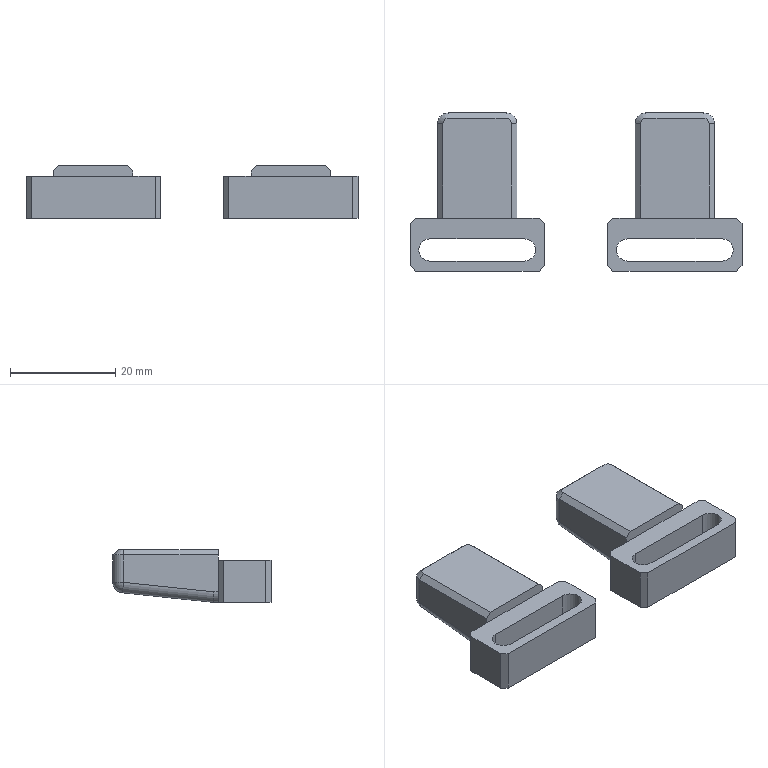NC program | NX | posted with a generic post | part box 63 x 30 x 10 mm
Lines 137 to 1195 of 24780:
(FIXED_CONTOUR , TOOL : D4R0.5)
N260 T16 M6
N262 G54
N264 G17 G0 G90 X-28.436 Y-13.585 B0. C0. S9500 M3
N266 G43 Z30. H16
N268 Z1.2
N270 G94 G1 Z-4.301 F1000.
N272 G3 X-28.236 Y-13.239 R0.4
N274 G1 Y-13.205 Z-4.212 F2500.
N276 X-28.242 Y-13.128 Z-4.201
N278 X-28.244 Y-12.729 Z-4.164
N280 X-28.245 Y1.946 Z-2.62
N282 X-28.246 Y2.589 Z-2.552
N284 X-28.245 Y2.666 Z-2.533
N286 X-28.243 Y2.712 Z-2.504
N288 X-28.238 Y2.806 Z-2.428
N290 X-28.236 Y2.911 Z-2.402
N292 Y2.92 Z-2.427
N294 Y2.921 Z-2.368
N296 Z-2.37
N298 Y2.939 Z-2.373
N300 Y2.944 Z-2.365
N302 Y2.961 Z-2.371
N304 Y2.981 Z-2.369
N306 Y2.999 Z-2.393
N308 Z-2.388
N310 Z-2.393
N312 Y2.981 Z-2.369
N314 Y2.961 Z-2.371
N316 Y2.944 Z-2.365
N318 Y2.939 Z-2.373
N320 Y2.921 Z-2.37
N322 Z-2.368
N324 Y2.92 Z-2.427
N326 Y2.911 Z-2.402
N328 X-28.238 Y2.806 Z-2.428
N330 Y0.416 Z-2.693
N332 Y-0.584 Z-2.805
N334 Y-3.37 Z-3.107
N336 Y-12.729 Z-4.086
N338 Y-12.885 Z-4.117
N340 Y-13.128 Z-4.155
N342 Y-13.177 Z-4.208
N344 X-28.236 Y-13.205 Z-4.212
N346 Y-13.239 Z-4.301
N348 X-28.231 Y-13.303
N350 Y-13.271 Z-4.215
N352 Y-13.128 Z-4.06
N354 Y-13.016 Z-4.042
N356 Y-12.729 Z-3.986
N358 X-28.23 Y-3.169 Z-2.996
N360 Y0.846 Z-2.545
N362 Y2.806 Z-2.334
N364 Y2.959
N366 Y2.963 Z-2.345
N368 Y2.964 Z-2.312
N370 Y2.982 Z-2.32
N372 Y2.991 Z-2.319
N374 Y2.999 Z-2.329
N376 X-28.226 Z-2.279
N378 X-28.221 Z-2.254
N380 Y2.94 Z-2.257
N382 Y0.251 Z-2.543
N384 Y-3.331 Z-2.934
N386 X-28.222 Y-11.136 Z-3.744
N388 Y-12.729 Z-3.91
N390 Y-13.128 Z-3.96
N392 Y-13.163 Z-3.981
N394 Y-13.383 Z-4.219
N396 Y-13.412 Z-4.301
N398 X-28.212 Y-13.528
N400 Y-13.526 Z-4.287
N402 Y-13.505 Z-4.224
N404 Y-13.293 Z-3.99
N406 Y-13.128 Z-3.89
N408 Y-12.729 Z-3.842
N410 X-28.211 Y-11.506 Z-3.713
N412 Y-8.746 Z-3.421
N414 Y2.815 Z-2.214
N416 Y2.999 Z-2.203
N418 X-28.2 Z-2.139
N420 Z-2.147
N422 Y2.806 Z-2.158
N424 Y-10.443 Z-3.545
N426 X-28.201 Y-12.434 Z-3.757
N428 Y-12.823 Z-3.798
N430 Y-13.128 Z-3.827
N432 Y-13.204 Z-3.859
N434 Y-13.436 Z-4.
N436 Y-13.526 Z-4.1
N438 Y-13.564 Z-4.2
N440 Y-13.576 Z-4.224
N442 Y-13.588 Z-4.301
N444 X-28.186 Y-13.667
N446 Y-13.655 Z-4.223
N448 Y-13.624 Z-4.16
N450 Y-13.563 Z-4.001
N452 Y-13.526 Z-3.952
N454 Y-13.405 Z-3.878
N456 Y-13.128 Z-3.761
N458 Y-12.965 Z-3.745
N460 Y-12.59 Z-3.705
N462 Y-5.957 Z-3.004
N464 X-28.185 Y2.806 Z-2.083
N466 Y2.999 Z-2.074
N468 Z-2.068
N470 X-28.167 Y2.998 Z-1.981
N472 Y2.806 Z-2.
N474 X-28.168 Y-12.729 Z-3.641
N476 Y-13.128 Z-3.68
N478 Y-13.155 Z-3.689
N480 Y-13.526 Z-3.844
N482 Y-13.555 Z-3.871
N484 Y-13.57 Z-3.882
N486 Y-13.654 Z-3.991
N488 Y-13.699 Z-4.11
N490 Y-13.754 Z-4.222
N492 Y-13.766 Z-4.301
N494 X-28.15 Y-13.865
N496 Y-13.853 Z-4.22
N498 Y-13.775 Z-4.06
N500 Y-13.744 Z-3.981
N502 Y-13.699 Z-3.92
N504 Y-13.653 Z-3.866
N506 Y-13.609 Z-3.835
N508 X-28.149 Y-13.526 Z-3.756
N510 Y-13.451 Z-3.724
N512 Y-13.128 Z-3.622
N514 Y-11.534 Z-3.456
N516 Y-3.368 Z-2.594
N518 Y2.998 Z-1.921
N520 X-28.129 Z-1.856
N522 Y-9.543 Z-3.183
N524 Y-13.128 Z-3.558
N526 Y-13.401 Z-3.645
N528 X-28.13 Y-13.526 Z-3.68
N530 Y-13.586 Z-3.717
N532 Y-13.668 Z-3.795
N534 Y-13.744 Z-3.849
N536 Y-13.823 Z-3.942
N538 Y-13.843 Z-3.97
N540 Y-13.857 Z-4.005
N542 Y-13.925 Z-4.143
N544 Y-13.948 Z-4.22
N546 Y-13.955 Z-4.3
N548 X-28.107 Y-14.03 Z-4.301
N550 Y-14.023 Z-4.222
N552 Y-14.01 Z-4.173
N554 Y-13.942 Z-3.957
N556 Y-13.925 Z-3.925
N558 Y-13.844 Z-3.831
N560 Y-13.734 Z-3.751
N562 Y-13.673 Z-3.693
N564 Y-13.526 Z-3.602
N566 Y-13.219 Z-3.517
N568 Y-13.128 Z-3.488
N570 Y-7.7 Z-2.92
N572 Y2.998 Z-1.785
N574 X-28.087 Y2.999 Z-1.74
N576 X-28.079 Z-1.717
N578 Z-1.722
N580 Y2.935 Z-1.723
N582 Y2.806 Z-1.732
N584 X-28.08 Y-9.144 Z-2.996
N586 Y-13.128 Z-3.412
N588 Y-13.526 Z-3.507
N590 Y-13.779 Z-3.664
N592 Y-13.814 Z-3.697
N594 Y-13.925 Z-3.776
N596 Y-13.961 Z-3.822
N598 Y-14.042 Z-3.973
N600 Y-14.091 Z-4.129
N602 Y-14.116 Z-4.224
N604 Y-14.123 Z-4.301
N606 X-28.052 Y-14.219
N608 Y-14.211 Z-4.226
N610 Y-14.174 Z-4.084
N612 Y-14.143 Z-3.984
N614 Y-14.114 Z-3.925
N616 Y-14.067 Z-3.841
N618 Y-14.032 Z-3.792
N620 Y-13.925 Z-3.66
N622 Y-13.89 Z-3.633
N624 Y-13.828 Z-3.595
N626 Y-13.569 Z-3.453
N628 Y-13.526 Z-3.432
N630 Y-13.331 Z-3.389
N632 Y-13.128 Z-3.34
N634 Y-6.5 Z-2.644
N636 X-28.051 Y2.806 Z-1.663
N638 Y2.87 Z-1.658
N640 Y2.999 Z-1.656
N642 Z-1.634
N644 X-28.023 Z-1.581
N646 Z-1.591
N648 Y2.809 Z-1.593
N650 X-28.024 Y-13.128 Z-3.269
N652 Y-13.526 Z-3.358
N654 Y-13.612 Z-3.399
N656 Y-13.698 Z-3.444
N658 Y-13.945 Z-3.581
N660 Y-13.986 Z-3.618
N662 Y-14.112 Z-3.775
N664 Y-14.174 Z-3.86
N666 Y-14.201 Z-3.909
N668 Y-14.244 Z-3.995
N670 Y-14.258 Z-4.039
N672 Y-14.307 Z-4.229
N674 Y-14.314 Z-4.3
N676 X-27.993 Y-14.399 Z-4.301
N678 Y-14.395 Z-4.24
N680 Y-14.386 Z-4.17
N682 Y-14.35 Z-4.015
N684 Y-14.323 Z-3.947
N686 Y-14.289 Z-3.88
N688 Y-14.199 Z-3.756
N690 Y-14.136 Z-3.679
N692 Y-14.083 Z-3.61
N694 Y-14.03 Z-3.559
N696 Y-13.977 Z-3.515
N698 Y-13.791 Z-3.41
N700 Y-13.658 Z-3.342
N702 Y-13.592 Z-3.309
N704 Y-13.526 Z-3.286
N706 Y-13.208 Z-3.217
N708 Y2.888 Z-1.522
N710 Y2.999 Z-1.521
N712 X-27.96 Z-1.445
N714 Y2.973
N716 X-27.961 Y-13.128 Z-3.142
N718 Y-13.297 Z-3.161
N720 Y-13.526 Z-3.213
N722 Y-13.692 Z-3.271
N724 Y-13.925 Z-3.392
N726 Y-14.012 Z-3.444
N728 Y-14.1 Z-3.516
N730 Y-14.188 Z-3.6
N732 Y-14.323 Z-3.778
N734 Y-14.389 Z-3.883
N736 Y-14.438 Z-4.003
N738 Y-14.457 Z-4.057
N740 Y-14.466 Z-4.096
N742 Y-14.487 Z-4.264
N744 Y-14.489 Z-4.301
N746 X-27.95 Y-14.519
N748 X-27.921 Y-14.581
N750 Y-14.578 Z-4.247
N752 Y-14.561 Z-4.117
N754 Y-14.549 Z-4.053
N756 Y-14.522 Z-3.976
N758 Y-14.484 Z-3.88
N760 Y-14.47 Z-3.853
N762 Y-14.389 Z-3.726
N764 Y-14.323 Z-3.63
N766 Y-14.28 Z-3.573
N768 Y-14.18 Z-3.477
N770 Y-14.109 Z-3.418
N772 Y-14.066 Z-3.389
N774 Y-13.996 Z-3.344
N776 Y-13.925 Z-3.302
N778 Y-13.782 Z-3.228
N780 Y-13.526 Z-3.138
N782 Y-13.383 Z-3.105
N784 Y-13.271 Z-3.088
N786 Y2.944 Z-1.378
N788 Y2.999 Z-1.376
N790 X-27.894 Z-1.333
N792 X-27.879 Z-1.306
N794 Z-1.311
N796 Y2.863 Z-1.316
N798 X-27.88 Y-13.188 Z-3.006
N800 Y-13.466 Z-3.05
N802 Y-13.526 Z-3.064
N804 Y-13.864 Z-3.183
N806 Y-13.925 Z-3.214
N808 Y-14.128 Z-3.342
N810 Y-14.233 Z-3.415
N812 Y-14.263 Z-3.44
N814 Y-14.323 Z-3.498
N816 Y-14.363 Z-3.547
N818 Y-14.388 Z-3.58
N820 Y-14.486 Z-3.722
N822 Y-14.543 Z-3.813
N824 Y-14.578 Z-3.877
N826 Y-14.601 Z-3.935
N828 Y-14.633 Z-4.026
N830 Y-14.661 Z-4.184
N832 Y-14.668 Z-4.233
N834 Y-14.671 Z-4.301
N836 X-27.857 Y-14.721
N838 X-27.837 Y-14.757
N840 Y-14.753 Z-4.223
N842 Y-14.718 Z-3.999
N844 Y-14.675 Z-3.875
N846 Y-14.618 Z-3.771
N848 Y-14.585 Z-3.719
N850 Y-14.528 Z-3.636
N852 Y-14.449 Z-3.53
N854 Y-14.356 Z-3.419
N856 Y-14.323 Z-3.386
N858 Y-14.192 Z-3.294
N860 Y-13.974 Z-3.156
N862 Y-13.925 Z-3.129
N864 Y-13.575 Z-3.006
N866 Y-13.526 Z-2.991
N868 Y-13.128 Z-2.929
N870 Y2.832 Z-1.251
N872 Y2.999 Z-1.244
N874 Z-1.238
N876 X-27.792 Z-1.175
N878 Y2.918 Z-1.178
N880 X-27.793 Y-13.128 Z-2.864
N882 Y-13.241 Z-2.885
N884 Y-13.354 Z-2.898
N886 Y-13.526 Z-2.925
N888 Y-13.752 Z-2.991
N890 Y-13.925 Z-3.053
N892 Y-14.15 Z-3.176
N894 Y-14.258 Z-3.244
N896 Y-14.323 Z-3.29
N898 Y-14.424 Z-3.385
N900 Y-14.476 Z-3.438
N902 Y-14.538 Z-3.513
N904 Y-14.688 Z-3.715
N906 Y-14.721 Z-3.773
N908 Y-14.764 Z-3.871
N910 Y-14.799 Z-3.995
N912 Y-14.834 Z-4.221
N914 Y-14.838 Z-4.301
N916 X-27.746 Y-14.925
N918 Y-14.921 Z-4.219
N920 Y-14.884 Z-3.992
N922 Y-14.848 Z-3.866
N924 Y-14.828 Z-3.824
N926 Y-14.779 Z-3.71
N928 Y-14.721 Z-3.611
N930 Y-14.634 Z-3.494
N932 Y-14.605 Z-3.459
N934 X-27.745 Y-14.509 Z-3.362
N936 Y-14.331 Z-3.195
N938 Y-14.323 Z-3.188
N940 Y-13.925 Z-2.972
N942 Y-13.526 Z-2.854
N944 Y-13.336 Z-2.833
N946 Y-13.128 Z-2.795
N948 Y2.998 Z-1.102
N950 X-27.697 Y2.999 Z-1.044
N952 Y-13.128 Z-2.738
N954 Y-13.337 Z-2.763
N956 Y-13.431 Z-2.78
N958 Y-13.526 Z-2.791
N960 Y-13.735 Z-2.847
N962 Y-13.925 Z-2.903
N964 Y-14.133 Z-3.002
N966 Y-14.323 Z-3.106
N968 Y-14.427 Z-3.185
N970 Y-14.492 Z-3.241
N972 Y-14.594 Z-3.338
N974 Y-14.728 Z-3.474
N976 Y-14.863 Z-3.705
N978 Y-14.9 Z-3.791
N980 Y-14.934 Z-3.861
N982 Y-14.971 Z-3.988
N984 Y-15.009 Z-4.217
N986 Y-15.012 Z-4.301
N988 X-27.649 Y-15.1
N990 Y-15.096 Z-4.215
N992 Y-15.057 Z-3.985
N994 Y-15.02 Z-3.856
N996 Y-14.971 Z-3.758
N998 Y-14.947 Z-3.7
N1000 Y-14.825 Z-3.491
N1002 Y-14.791 Z-3.441
N1004 Y-14.721 Z-3.356
N1006 Y-14.647 Z-3.283
N1008 Y-14.523 Z-3.176
N1010 Y-14.324 Z-3.024
N1012 Y-13.925 Z-2.835
N1014 Y-13.526 Z-2.728
N1016 Y-13.128 Z-2.68
N1018 X-27.648 Y2.999 Z-0.986
N1020 Z-0.984
N1022 X-27.599 Z-0.926
N1024 Y-13.128 Z-2.621
N1026 Y-13.526 Z-2.669
N1028 Y-13.627 Z-2.691
N1030 Y-13.824 Z-2.744
N1032 Y-13.925 Z-2.773
N1034 Y-14.025 Z-2.81
N1036 Y-14.323 Z-2.952
N1038 Y-14.423 Z-3.013
N1040 Y-14.623 Z-3.166
N1042 Y-14.721 Z-3.251
N1044 Y-14.791 Z-3.327
N1046 Y-14.856 Z-3.406
N1048 Y-14.923 Z-3.502
N1050 Y-15.033 Z-3.694
N1052 Y-15.046 Z-3.723
N1054 Y-15.108 Z-3.851
N1056 Y-15.148 Z-4.001
N1058 Y-15.171 Z-4.15
N1060 Y-15.178 Z-4.23
N1062 Y-15.181 Z-4.301
N1064 X-27.547 Y-15.263
N1066 Y-15.261 Z-4.25
N1068 Y-15.243 Z-4.06
N1070 Y-15.192 Z-3.852
N1072 Y-15.12 Z-3.681
N1074 Y-15.023 Z-3.511
N1076 Y-14.923 Z-3.369
N1078 Y-14.721 Z-3.152
N1080 Y-14.528 Z-3.002
N1082 Y-14.323 Z-2.877
N1084 Y-14.127 Z-2.783
N1086 Y-13.925 Z-2.709
N1088 Y-13.728 Z-2.652
N1090 Y-13.526 Z-2.609
N1092 Y-13.128 Z-2.56
N1094 X-27.546 Y2.998 Z-0.864
N1096 X-27.487 Y2.999 Z-0.808
N1098 X-27.488 Y-13.251 Z-2.518
N1100 Y-13.526 Z-2.552
N1102 Y-13.787 Z-2.607
N1104 Y-13.925 Z-2.647
N1106 Y-14.185 Z-2.741
N1108 Y-14.323 Z-2.808
N1110 Y-14.446 Z-2.877
N1112 Y-14.645 Z-3.
N1114 Y-14.721 Z-3.059
N1116 Y-14.844 Z-3.178
N1118 Y-14.982 Z-3.326
N1120 Y-15.043 Z-3.399
N1122 Y-15.081 Z-3.454
N1124 Y-15.12 Z-3.521
N1126 Y-15.198 Z-3.666
N1128 Y-15.268 Z-3.836
N1130 Y-15.312 Z-4.008
N1132 Y-15.334 Z-4.168
N1134 Y-15.34 Z-4.234
N1136 Y-15.343 Z-4.301
N1138 X-27.428 Y-15.424
N1140 Y-15.42 Z-4.229
N1142 Y-15.381 Z-3.955
N1144 Y-15.346 Z-3.82
N1146 Y-15.273 Z-3.644
N1148 Y-15.184 Z-3.479
N1150 Y-15.144 Z-3.409
N1152 Y-15.12 Z-3.376
N1154 Y-15.041 Z-3.283
N1156 Y-14.963 Z-3.198
N1158 Y-14.882 Z-3.122
N1160 Y-14.75 Z-2.994
N1162 Y-14.721 Z-2.97
N1164 Y-14.565 Z-2.873
N1166 Y-14.323 Z-2.737
N1168 Y-14.245 Z-2.699
N1170 Y-13.925 Z-2.585
N1172 Y-13.846 Z-2.562
N1174 Y-13.526 Z-2.495
N1176 Y-13.128 Z-2.449
N1178 Y2.999 Z-0.752
N1180 X-27.367 Z-0.695
N1182 X-27.368 Y-13.128 Z-2.392
N1184 Y-13.526 Z-2.437
N1186 Y-13.906 Z-2.517
N1188 Y-14.305 Z-2.656
N1190 Y-14.685 Z-2.869
N1192 Y-14.721 Z-2.892
N1194 Y-14.884 Z-3.028
N1196 Y-14.962 Z-3.105
N1198 Y-15.083 Z-3.219
N1200 Y-15.12 Z-3.26
N1202 Y-15.213 Z-3.387
N1204 Y-15.351 Z-3.629
N1206 Y-15.428 Z-3.829
N1208 Y-15.465 Z-3.976
N1210 Y-15.501 Z-4.239
N1212 Y-15.503 Z-4.301
N1214 X-27.307 Y-15.575
N1216 Y-15.569 Z-4.197
N1218 Y-15.545 Z-3.993
N1220 Y-15.514 Z-3.844
N1222 Y-15.44 Z-3.654
N1224 Y-15.393 Z-3.564
N1226 Y-15.283 Z-3.365
N1228 Y-15.161 Z-3.204
N1230 Y-15.12 Z-3.159
N1232 Y-15.006 Z-3.051
N1234 Y-14.911 Z-2.969
N1236 Y-14.764 Z-2.848
N1238 Y-14.721 Z-2.821
N1240 Y-14.409 Z-2.644
N1242 Y-14.366 Z-2.622
N1244 Y-14.323 Z-2.603
N1246 Y-13.967 Z-2.479
N1248 Y-13.925 Z-2.467
N1250 Y-13.612 Z-2.402
N1252 Y-13.526 Z-2.386
N1254 Y-13.128 Z-2.342
N1256 X-27.306 Y2.999 Z-0.644
N1258 X-27.241 Y3. Z-0.595
N1260 X-27.242 Y-13.343 Z-2.315
N1262 Y-13.526 Z-2.335
N1264 Y-13.741 Z-2.375
N1266 Y-13.925 Z-2.413
N1268 Y-14.032 Z-2.443
N1270 Y-14.323 Z-2.543
N1272 Y-14.43 Z-2.589
N1274 Y-14.538 Z-2.646
N1276 Y-14.721 Z-2.749
N1278 Y-14.829 Z-2.817
N1280 Y-14.997 Z-2.956
N1282 Y-15.125 Z-3.066
N1284 Y-15.224 Z-3.172
N1286 Y-15.339 Z-3.327
N1288 Y-15.379 Z-3.389
N1290 Y-15.445 Z-3.508
N1292 Y-15.53 Z-3.676
N1294 Y-15.588 Z-3.847
N1296 Y-15.624 Z-4.02
N1298 Y-15.638 Z-4.139
N1300 Y-15.646 Z-4.244
N1302 Y-15.648 Z-4.301
N1304 X-27.177 Y-15.722
N1306 Y-15.72 Z-4.246
N1308 Y-15.703 Z-4.046
N1310 Y-15.662 Z-3.848
N1312 Y-15.604 Z-3.678
N1314 Y-15.518 Z-3.493
N1316 Y-15.477 Z-3.417
N1318 Y-15.395 Z-3.288
N1320 Y-15.291 Z-3.149
N1322 Y-15.171 Z-3.02
N1324 Y-15.084 Z-2.943
N1326 Y-14.894 Z-2.786
N1328 Y-14.721 Z-2.677
N1330 Y-14.668 Z-2.647
N1332 Y-14.495 Z-2.557
N1334 Y-14.323 Z-2.482
N1336 Y-14.097 Z-2.406
N1338 Y-13.925 Z-2.358
N1340 Y-13.526 Z-2.284
N1342 X-27.176 Y-11.229 Z-2.041
N1344 Y3. Z-0.545
N1346 X-27.144 Z-0.522
N1348 X-27.108 Y3.002 Z-0.499
N1350 Y-13.526 Z-2.237
N1352 Y-13.609 Z-2.25
N1354 Y-13.925 Z-2.308
N1356 Y-14.165 Z-2.374
N1358 Y-14.323 Z-2.426
N1360 Y-14.563 Z-2.528
N1362 Y-14.721 Z-2.611
N1364 Y-14.962 Z-2.762
N1366 Y-15.12 Z-2.892
N1368 Y-15.235 Z-2.998
N1370 X-27.109 Y-15.36 Z-3.133
N1372 Y-15.459 Z-3.264
N1374 Y-15.549 Z-3.407
N1376 Y-15.581 Z-3.466
N1378 Y-15.668 Z-3.655
N1380 Y-15.729 Z-3.828
N1382 Y-15.742 Z-3.881
N1384 Y-15.769 Z-4.01
N1386 Y-15.785 Z-4.131
N1388 Y-15.793 Z-4.234
N1390 Y-15.795 Z-4.301
N1392 X-27.039 Y-15.865
N1394 Y-15.859 Z-4.182
N1396 Y-15.826 Z-3.931
N1398 Y-15.791 Z-3.793
N1400 Y-15.725 Z-3.612
N1402 Y-15.686 Z-3.528
N1404 Y-15.601 Z-3.369
N1406 Y-15.532 Z-3.256
N1408 Y-15.429 Z-3.121
N1410 Y-15.312 Z-2.992
N1412 Y-15.12 Z-2.816
N1414 Y-15.031 Z-2.743
N1416 Y-14.721 Z-2.549
N1418 Y-14.633 Z-2.503
N1420 Y-14.323 Z-2.373
N1422 Y-14.234 Z-2.344
N1424 Y-13.925 Z-2.261
N1426 Y-13.748 Z-2.229
N1428 Y-13.526 Z-2.193
N1430 X-27.038 Y3.005 Z-0.457
N1432 X-27.015 Y3.006 Z-0.442
N1434 X-27.016 Z-0.44
N1436 X-26.968 Y3.009 Z-0.413
N1438 Y-13.526 Z-2.148
N1440 Y-13.925 Z-2.214
N1442 Y-14.304 Z-2.314
N1444 Y-14.323 Z-2.32
N1446 Y-14.703 Z-2.477
N1448 Y-14.721 Z-2.487
N1450 Y-15.101 Z-2.724
N1452 Y-15.388 Z-2.986
N1454 Y-15.499 Z-3.108
N1456 Y-15.621 Z-3.278
N1458 X-26.969 Y-15.654 Z-3.332
N1460 Y-15.78 Z-3.569
N1462 Y-15.844 Z-3.749
N1464 Y-15.866 Z-3.82
N1466 Y-15.881 Z-3.881
N1468 Y-15.915 Z-4.062
N1470 Y-15.928 Z-4.239
N1472 Y-15.93 Z-4.301
N1474 X-26.894 Y-15.995
N1476 Y-15.993 Z-4.24
N1478 Y-15.984 Z-4.121
N1480 Y-15.976 Z-4.034
N1482 Y-15.942 Z-3.849
N1484 Y-15.896 Z-3.698
N1486 Y-15.881 Z-3.654
N1488 Y-15.826 Z-3.521
N1490 Y-15.709 Z-3.295
N1492 Y-15.569 Z-3.097
N1494 Y-15.518 Z-3.033
N1496 Y-15.469 Z-2.979
N1498 Y-15.175 Z-2.711
N1500 Y-15.12 Z-2.671
N1502 Y-14.777 Z-2.458
N1504 Y-14.721 Z-2.431
N1506 Y-14.378 Z-2.291
N1508 Y-14.323 Z-2.272
N1510 Y-13.98 Z-2.182
N1512 Y-13.925 Z-2.17
N1514 Y-13.637 Z-2.124
N1516 Y-13.526 Z-2.108
N1518 X-26.893 Y3.019 Z-0.372
N1520 X-26.868 Y3.021 Z-0.358
N1522 X-26.818 Y3.033 Z-0.331
N1524 X-26.819 Y-13.526 Z-2.07
N1526 Y-13.787 Z-2.107
N1528 Y-13.925 Z-2.129
N1530 Y-14.055 Z-2.157
N1532 Y-14.323 Z-2.226
N1534 Y-14.453 Z-2.27
N1536 Y-14.583 Z-2.321
N1538 Y-14.721 Z-2.378
N1540 Y-14.851 Z-2.442
N1542 Y-14.982 Z-2.52
N1544 Y-15.12 Z-2.606
N1546 Y-15.25 Z-2.701
N1548 Y-15.518 Z-2.943
N1550 Y-15.64 Z-3.089
N1552 Y-15.765 Z-3.273
N1554 Y-15.82 Z-3.369
N1556 Y-15.873 Z-3.472
N1558 Y-15.957 Z-3.677
N1560 Y-16.008 Z-3.846
N1562 Y-16.037 Z-4.008
N1564 Y-16.059 Z-4.241
N1566 Y-16.061 Z-4.301
N1568 X-26.743 Y-16.126
N1570 Y-16.124 Z-4.238
N1572 Y-16.099 Z-3.986
N1574 Y-16.073 Z-3.845
N1576 Y-16.021 Z-3.67
N1578 Y-15.916 Z-3.417
N1580 Y-15.823 Z-3.254
N1582 Y-15.723 Z-3.108
N1584 Y-15.622 Z-2.977
N1586 Y-15.518 Z-2.865
N1588 Y-15.325 Z-2.692
N1590 Y-15.12 Z-2.542
N1592 Y-14.927 Z-2.426
N1594 Y-14.721 Z-2.325
N1596 Y-14.528 Z-2.25
N1598 Y-14.323 Z-2.18
N1600 Y-14.13 Z-2.132
N1602 Y-13.925 Z-2.088
N1604 Y-13.526 Z-2.032
N1606 Y1.539 Z-0.449
N1608 Y3.047 Z-0.29
N1610 X-26.685 Y3.061 Z-0.265
N1612 X-26.663 Y3.068 Z-0.253
N1614 Y3.067 Z-0.255
N1616 X-26.664 Y-13.526 Z-1.999
N1618 Y-13.697 Z-2.021
N1620 Y-13.925 Z-2.053
N1622 Y-14.209 Z-2.112
N1624 Y-14.323 Z-2.14
N1626 Y-14.608 Z-2.235
N1628 Y-14.721 Z-2.279
N1630 Y-15.006 Z-2.418
N1632 Y-15.12 Z-2.486
N1634 Y-15.205 Z-2.546
N1636 Y-15.404 Z-2.693
N1638 Y-15.518 Z-2.795
N1640 Y-15.682 Z-2.969
N1642 Y-15.803 Z-3.123
N1644 Y-15.902 Z-3.27
N1646 Y-15.916 Z-3.295
N1648 Y-15.98 Z-3.426
N1650 Y-16.06 Z-3.62
N1652 Y-16.095 Z-3.723
N1654 Y-16.132 Z-3.849
N1656 Y-16.161 Z-4.009
N1658 Y-16.179 Z-4.189
N1660 Y-16.185 Z-4.301
N1662 X-26.584 Y-16.244
N1664 Y-16.235 Z-4.139
N1666 Y-16.224 Z-4.033
N1668 Y-16.191 Z-3.854
N1670 Y-16.141 Z-3.686
N1672 Y-16.099 Z-3.57
N1674 Y-16.04 Z-3.425
N1676 Y-15.96 Z-3.263
N1678 Y-15.916 Z-3.188
N1680 Y-15.865 Z-3.116
N1682 Y-15.741 Z-2.962
N1684 Y-15.6 Z-2.809
N1686 Y-15.518 Z-2.724
N1688 Y-15.484 Z-2.693
N1690 Y-15.285 Z-2.547
N1692 Y-15.12 Z-2.431
N1694 Y-15.085 Z-2.41
N1696 Y-14.721 Z-2.234
N1698 Y-14.653 Z-2.209
N1700 Y-14.323 Z-2.101
N1702 Y-14.255 Z-2.085
N1704 Y-13.925 Z-2.017
N1706 Y-13.526 Z-1.966
N1708 X-26.583 Y3.088 Z-0.219
N1710 X-26.55 Y3.096 Z-0.205
N1712 X-26.503 Y3.112 Z-0.188
N1714 X-26.504 Y-10.906 Z-1.662
N1716 Y-13.617 Z-1.947
N1718 Y-13.925 Z-1.986
N1720 Y-14.015 Z-2.003
N1722 Y-14.323 Z-2.066
N1724 Y-14.368 Z-2.077
N1726 Y-14.721 Z-2.192
N1728 Y-14.767 Z-2.21
N1730 Y-15.12 Z-2.38
N1732 Y-15.165 Z-2.407
N1734 Y-15.364 Z-2.547
N1736 Y-15.518 Z-2.66
N1738 Y-15.563 Z-2.7
N1740 Y-15.679 Z-2.82
N1742 Y-15.801 Z-2.954
N1744 Y-15.939 Z-3.128
N1746 Y-16.013 Z-3.251
N1748 Y-16.1 Z-3.425
N1750 Y-16.139 Z-3.52
N1752 Y-16.2 Z-3.691
N1754 Y-16.251 Z-3.859
N1756 Y-16.287 Z-4.057
N1758 Y-16.303 Z-4.301
N1760 X-26.423 Y-16.356
N1762 Y-16.347 Z-4.133
N1764 Y-16.339 Z-4.04
N1766 Y-16.311 Z-3.863
N1768 Y-16.26 Z-3.697
N1770 Y-16.179 Z-3.469
N1772 Y-16.16 Z-3.424
N1774 Y-16.067 Z-3.239
N1776 Y-16.042 Z-3.198
N1778 Y-15.979 Z-3.099
N1780 Y-15.916 Z-3.014
N1782 Y-15.862 Z-2.946
N1784 Y-15.681 Z-2.749
N1786 Y-15.644 Z-2.711
N1788 Y-15.518 Z-2.601
N1790 Y-15.445 Z-2.547
N1792 Y-15.246 Z-2.407
N1794 Y-15.12 Z-2.333
N1796 Y-14.847 Z-2.202
N1798 Y-14.721 Z-2.153
N1800 Y-14.449 Z-2.065
N1802 Y-14.323 Z-2.033
N1804 Y-14.177 Z-2.003
N1806 Y-13.925 Z-1.958
N1808 Y-13.526 Z-1.91
N1810 Y-5.034 Z-1.02
N1812 X-26.422 Y3.137 Z-0.16
N1814 Y3.138 Z-0.158
N1816 X-26.339 Y3.165 Z-0.129
N1818 X-26.34 Y-7.446 Z-1.249
N1820 Y-13.545 Z-1.886
N1822 Y-13.944 Z-1.933
N1824 Y-14.323 Z-2.001
N1826 Y-14.532 Z-2.053
N1828 Y-14.721 Z-2.115
N1830 Y-14.93 Z-2.195
N1832 Y-15.124 Z-2.288
N1834 Y-15.328 Z-2.409
N1836 Y-15.523 Z-2.545
N1838 Y-15.727 Z-2.724
N1840 Y-15.921 Z-2.938
N1842 Y-16.021 Z-3.071
N1844 Y-16.125 Z-3.235
N1846 Y-16.224 Z-3.433
N1848 Y-16.32 Z-3.702
N1850 Y-16.362 Z-3.867
N1852 Y-16.383 Z-3.997
N1854 Y-16.404 Z-4.236
N1856 Y-16.407 Z-4.301
N1858 X-26.255 Y-16.452
N1860 Y-16.45 Z-4.23
N1862 Y-16.43 Z-3.997
N1864 Y-16.409 Z-3.868
N1866 Y-16.368 Z-3.706
N1868 Y-16.31 Z-3.517
N1870 Y-16.262 Z-3.4
N1872 Y-16.21 Z-3.298
N1874 Y-16.163 Z-3.213
N1876 Y-16.063 Z-3.056
N1878 Y-15.916 Z-2.862
N1880 Y-15.812 Z-2.748
N1882 Y-15.565 Z-2.53
N1884 Y-15.518 Z-2.491
N1886 Y-15.413 Z-2.418
N1888 Y-15.12 Z-2.245
N1890 Y-15.015 Z-2.196
N1892 Y-14.721 Z-2.081
N1894 Y-14.617 Z-2.047
N1896 Y-14.323 Z-1.973
N1898 Y-14.114 Z-1.936
N1900 Y-13.925 Z-1.906
N1902 Y-13.526 Z-1.862
N1904 X-26.254 Y-4.858 Z-0.953
N1906 Y2.99 Z-0.127
N1908 Y3.197 Z-0.102
N1910 X-26.233 Y3.206 Z-0.096
N1912 X-26.166 Y3.236 Z-0.08
N1914 Y2.836 Z-0.121
N1916 X-26.167 Y-13.925 Z-1.883
N1918 Y-14.323 Z-1.945
N1920 Y-14.721 Z-2.047
N1922 Y-15.102 Z-2.196
N1924 Y-15.211 Z-2.256
N1926 Y-15.501 Z-2.427
N1928 Y-15.518 Z-2.439
N1930 Y-15.609 Z-2.514
N1932 Y-15.899 Z-2.772
N1934 Y-15.916 Z-2.791
N1936 Y-16.107 Z-3.041
N1938 Y-16.206 Z-3.199
N1940 Y-16.306 Z-3.379
N1942 Y-16.356 Z-3.512
N1944 Y-16.417 Z-3.709
N1946 Y-16.457 Z-3.87
N1948 Y-16.477 Z-3.996
N1950 Y-16.497 Z-4.224
N1952 Y-16.499 Z-4.301
N1954 X-26.079 Y-16.547
N1956 Y-16.545 Z-4.218
N1958 Y-16.525 Z-3.995
N1960 Y-16.506 Z-3.871
N1962 Y-16.467 Z-3.712
N1964 Y-16.4 Z-3.501
N1966 Y-16.367 Z-3.414
N1968 Y-16.341 Z-3.352
N1970 Y-16.315 Z-3.301
N1972 Y-16.25 Z-3.185
N1974 Y-16.151 Z-3.026
N1976 Y-15.987 Z-2.81
N1978 Y-15.916 Z-2.732
N1980 Y-15.653 Z-2.498
N1982 Y-15.588 Z-2.445
N1984 Y-15.518 Z-2.395
N1986 Y-15.254 Z-2.24
N1988 Y-15.19 Z-2.203
N1990 Y-15.12 Z-2.169
N1992 Y-14.792 Z-2.041
N1994 Y-14.721 Z-2.018
N1996 Y-14.393 Z-1.936
N1998 Y-14.323 Z-1.922
N2000 Y-14.065 Z-1.882
N2002 Y-13.925 Z-1.864
N2004 X-26.078 Y3.205 Z-0.065
N2006 Y3.274 Z-0.059
N2008 X-25.991 Y3.319 Z-0.037
N2010 Y3.124 Z-0.055
N2012 Y-13.925 Z-1.846
N2014 Y-14.24 Z-1.887
N2016 Y-14.323 Z-1.9
N2018 Y-14.481 Z-1.931
N2020 Y-14.721 Z-1.989
N2022 Y-14.879 Z-2.041
N2024 Y-15.12 Z-2.135
N2026 Y-15.277 Z-2.212
N2028 Y-15.518 Z-2.351
N2030 Y-15.676 Z-2.465
N2032 Y-15.916 Z-2.677
N2034 Y-16.074 Z-2.852
N2036 Y-16.194 Z-3.011
N2038 Y-16.294 Z-3.17
N2040 Y-16.374 Z-3.324
N2042 Y-16.433 Z-3.462
N2044 Y-16.516 Z-3.715
N2046 Y-16.556 Z-3.886
N2048 Y-16.573 Z-3.995
N2050 Y-16.592 Z-4.212
N2052 Y-16.594 Z-4.301
N2054 X-25.944 Y-16.619
N2056 X-25.902 Y-16.638
N2058 Y-16.634 Z-4.185
N2060 Y-16.617 Z-3.999
N2062 Y-16.598 Z-3.879
N2064 Y-16.554 Z-3.699
N2066 Y-16.482 Z-3.478
N2068 Y-16.404 Z-3.298
N2070 Y-16.339 Z-3.169
N2072 Y-16.315 Z-3.126
N2074 Y-16.239 Z-3.005
N2076 Y-16.139 Z-2.874
N2078 Y-16.115 Z-2.845
N2080 Y-15.916 Z-2.626
N2082 Y-15.765 Z-2.492
N2084 Y-15.717 Z-2.455
N2086 Y-15.518 Z-2.312
N2088 Y-15.343 Z-2.212
N2090 Y-15.12 Z-2.104
N2092 Y-14.968 Z-2.044
N2094 Y-14.721 Z-1.965
N2096 Y-14.546 Z-1.924
N2098 Y-14.323 Z-1.881
N2100 Y-14.02 Z-1.842
N2102 X-25.901 Y3.205 Z-0.032
N2104 Y3.306 Z-0.023
N2106 Y3.334
N2108 Y3.364 Z-0.018
N2110 X-25.837 Y3.396 Z-0.006
N2112 X-25.81 Y3.414 Z-0.001
N2114 Y3.326 Z-0.017
N2116 Y3.245
N2118 Y-1.376 Z-0.501
N2120 X-25.811 Y-14.202 Z-1.849
N2122 Y-14.323 Z-1.864
N2124 Y-14.591 Z-1.915
N2126 Y-14.721 Z-1.944
N2128 Y-14.791 Z-1.964
N2130 Y-15.059 Z-2.051
N2132 Y-15.12 Z-2.075
N2134 Y-15.388 Z-2.206
N2136 Y-15.457 Z-2.242
N2138 Y-15.518 Z-2.278
N2140 Y-15.587 Z-2.324
N2142 Y-15.717 Z-2.418
N2144 Y-15.786 Z-2.47
N2146 Y-15.856 Z-2.526
N2148 Y-15.916 Z-2.579
N2150 Y-15.986 Z-2.65
N2152 Y-16.115 Z-2.795
N2154 Y-16.185 Z-2.878
N2156 Y-16.284 Z-3.007
N2158 Y-16.315 Z-3.056
N2160 Y-16.384 Z-3.18
N2162 Y-16.433 Z-3.275
N2164 Y-16.516 Z-3.465
N2166 Y-16.582 Z-3.665
N2168 Y-16.6 Z-3.728
N2170 Y-16.638 Z-3.889
N2172 Y-16.664 Z-4.049
N2174 Y-16.672 Z-4.139
N2176 Y-16.678 Z-4.242
N2178 Y-16.679 Z-4.301
N2180 X-25.72 Y-16.719
N2182 Y-16.708 Z-4.085
N2184 Y-16.678 Z-3.899
N2186 Y-16.639 Z-3.735
N2188 Y-16.611 Z-3.632
N2190 Y-16.579 Z-3.533
N2192 Y-16.55 Z-3.453
N2194 Y-16.461 Z-3.252
N2196 Y-16.429 Z-3.19
N2198 Y-16.33 Z-3.013
N2200 Y-16.315 Z-2.991
N2202 Y-16.23 Z-2.882
N2204 Y-16.115 Z-2.744
N2206 Y-16.031 Z-2.65
N2208 Y-15.946 Z-2.563
N2210 Y-15.916 Z-2.535
N2212 Y-15.832 Z-2.467
N2214 Y-15.717 Z-2.38
N2216 Y-15.633 Z-2.319
N2218 Y-15.518 Z-2.244
N2220 Y-15.433 Z-2.199
N2222 Y-15.15 Z-2.06
N2224 Y-15.09 Z-2.038
N2226 Y-14.836 Z-1.956
N2228 Y-14.721 Z-1.924
N2230 Y-14.437 Z-1.868
N2232 Y-14.323 Z-1.849
N2234 X-25.719 Y3.143 Z-0.014
N2236 Y3.22 Z-0.01
N2238 Y3.317 Z-0.011
N2240 Y3.373 Z0.
N2242 Y3.453
N2244 X-25.664 Y3.473
N2246 X-25.635 Y3.468
N2248 X-25.626 Y3.452
N2250 Y3.333
N2252 Y3.308 Z-0.005
N2254 Y3.205
N2256 Y2.959 Z-0.021
N2258 X-25.627 Y-14.323 Z-1.837
N2260 Y-14.445 Z-1.853
N2262 Y-14.721 Z-1.905
N2264 Y-14.882 Z-1.948
N2266 Y-15.12 Z-2.025
N2268 Y-15.242 Z-2.074
N2270 Y-15.518 Z-2.213
N2272 Y-15.679 Z-2.315
N2274 Y-15.878 Z-2.464
N2276 Y-15.916 Z-2.495
N2278 Y-16.038 Z-2.61
N2280 Y-16.115 Z-2.693
N2282 Y-16.276 Z-2.886
N2284 Y-16.315 Z-2.936
N2286 Y-16.376 Z-3.025
N2288 Y-16.475 Z-3.2
N2290 Y-16.49 Z-3.229
N2292 Y-16.585 Z-3.44
N2294 Y-16.639 Z-3.598
N2296 Y-16.679 Z-3.742
N2298 Y-16.718 Z-3.907
N2300 Y-16.738 Z-4.049
N2302 Y-16.746 Z-4.157
N2304 Y-16.752 Z-4.301
N2306 X-25.534 Y-16.784
N2308 Y-16.782 Z-4.221
N2310 Y-16.766 Z-4.01
N2312 Y-16.747 Z-3.892
N2314 Y-16.713 Z-3.727
N2316 Y-16.671 Z-3.576
N2318 Y-16.617 Z-3.427
N2320 Y-16.518 Z-3.207
N2322 Y-16.418 Z-3.034
N2324 Y-16.315 Z-2.882
N2326 Y-16.131 Z-2.661
N2328 Y-15.924 Z-2.464
N2330 Y-15.717 Z-2.307
N2332 Y-15.518 Z-2.183
N2334 Y-15.319 Z-2.083
N2336 Y-15.12 Z-2.003
N2338 Y-14.92 Z-1.939
N2340 Y-14.721 Z-1.888
N2342 Y-14.53 Z-1.853
N2344 Y-14.307 Z-1.823
N2346 X-25.533 Y2.806 Z-0.025
N2348 Y3.19 Z-0.001
N2350 Y3.273 Z0.
N2352 X-25.485 Y3.196
N2354 X-25.439 Y3.137
N2356 Y3.095 Z-0.001
N2358 Y2.806 Z-0.019
N2360 Y2.696 Z-0.029
N2362 X-25.44 Y-14.323 Z-1.817
N2364 Y-14.577 Z-1.85
N2366 Y-14.776 Z-1.887
N2368 Y-14.975 Z-1.939
N2370 Y-15.174 Z-2.006